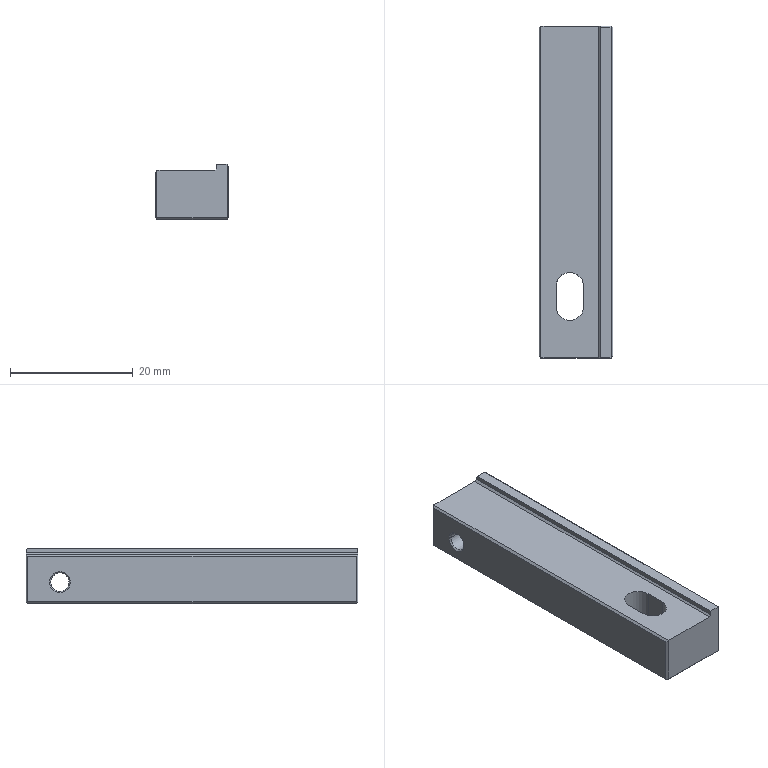Part | NX | 1 solid | 32 faces | box 12 x 54 x 9 mm | volume 4930 mm3 | plane 22 | cylinder 6 | cone 4 | commonest cylinder face diameters 2.5 x2 3 x2 4.5 x2
STEP:
#1=CARTESIAN_POINT('',(2266.8,144.7,-81.));
#2=VERTEX_POINT('',#1);
#3=CARTESIAN_POINT('',(2278.2,144.7,-81.));
#4=VERTEX_POINT('',#3);
#5=CARTESIAN_POINT('',(2272.5,144.7,-81.));
#6=DIRECTION('',(1.,0.,0.));
#7=VECTOR('',#6,1000.);
#8=LINE('',#5,#7);
#9=EDGE_CURVE('',#2,#4,#8,.T.);
#10=ORIENTED_EDGE('',*,*,#9,.T.);
#11=CARTESIAN_POINT('',(2278.2,91.3,-81.));
#12=VERTEX_POINT('',#11);
#13=CARTESIAN_POINT('',(2278.2,118.,-81.));
#14=DIRECTION('',(0.,-1.,0.));
#15=VECTOR('',#14,1000.);
#16=LINE('',#13,#15);
#17=EDGE_CURVE('',#4,#12,#16,.T.);
#18=ORIENTED_EDGE('',*,*,#17,.T.);
#19=CARTESIAN_POINT('',(2266.8,91.3,-81.));
#20=VERTEX_POINT('',#19);
#21=CARTESIAN_POINT('',(2272.5,91.3,-81.));
#22=DIRECTION('',(1.,0.,0.));
#23=VECTOR('',#22,1000.);
#24=LINE('',#21,#23);
#25=EDGE_CURVE('',#20,#12,#24,.T.);
#26=ORIENTED_EDGE('',*,*,#25,.F.);
#27=CARTESIAN_POINT('',(2266.8,118.,-81.));
#28=DIRECTION('',(0.,-1.,0.));
#29=VECTOR('',#28,1000.);
#30=LINE('',#27,#29);
#31=EDGE_CURVE('',#2,#20,#30,.T.);
#32=ORIENTED_EDGE('',*,*,#31,.F.);
#33=EDGE_LOOP('',(#10,#18,#26,#32));
#34=FACE_BOUND('',#33,.T.);
#35=CARTESIAN_POINT('',(2273.75,99.35,-81.));
#36=VERTEX_POINT('',#35);
#37=CARTESIAN_POINT('',(2269.25,99.35,-81.));
#38=VERTEX_POINT('',#37);
#39=CARTESIAN_POINT('',(2271.5,99.35,-81.));
#40=DIRECTION('',(0.,0.,-1.));
#41=DIRECTION('',(-1.,0.,0.));
#42=AXIS2_PLACEMENT_3D('',#39,#40,#41);
#43=CIRCLE('',#42,2.25);
#44=EDGE_CURVE('',#36,#38,#43,.T.);
#45=ORIENTED_EDGE('',*,*,#44,.F.);
#46=CARTESIAN_POINT('',(2273.75,102.65,-81.));
#47=VERTEX_POINT('',#46);
#48=CARTESIAN_POINT('',(2273.75,45.25,-81.));
#49=DIRECTION('',(0.,-1.,0.));
#50=VECTOR('',#49,1000.);
#51=LINE('',#48,#50);
#52=EDGE_CURVE('',#47,#36,#51,.T.);
#53=ORIENTED_EDGE('',*,*,#52,.F.);
#54=CARTESIAN_POINT('',(2269.25,102.65,-81.));
#55=VERTEX_POINT('',#54);
#56=CARTESIAN_POINT('',(2271.5,102.65,-81.));
#57=DIRECTION('',(0.,0.,-1.));
#58=DIRECTION('',(-1.,0.,0.));
#59=AXIS2_PLACEMENT_3D('',#56,#57,#58);
#60=CIRCLE('',#59,2.25);
#61=EDGE_CURVE('',#55,#47,#60,.T.);
#62=ORIENTED_EDGE('',*,*,#61,.F.);
#63=CARTESIAN_POINT('',(2269.25,45.25,-81.));
#64=DIRECTION('',(0.,1.,0.));
#65=VECTOR('',#64,1000.);
#66=LINE('',#63,#65);
#67=EDGE_CURVE('',#38,#55,#66,.T.);
#68=ORIENTED_EDGE('',*,*,#67,.F.);
#69=EDGE_LOOP('',(#45,#53,#62,#68));
#70=FACE_BOUND('',#69,.T.);
#71=CARTESIAN_POINT('',(2266.5,125.,-81.));
#72=DIRECTION('',(0.,0.,-1.));
#73=DIRECTION('',(0.,-1.,0.));
#74=AXIS2_PLACEMENT_3D('',#71,#72,#73);
#75=PLANE('',#74);
#76=ADVANCED_FACE('',(#34,#70),#75,.T.);
#77=CARTESIAN_POINT('',(2278.2,145.,-72.3));
#78=VERTEX_POINT('',#77);
#79=CARTESIAN_POINT('',(2276.5,145.,-72.3));
#80=VERTEX_POINT('',#79);
#81=CARTESIAN_POINT('',(2277.35,145.,-72.3));
#82=DIRECTION('',(-1.,0.,0.));
#83=VECTOR('',#82,1000.);
#84=LINE('',#81,#83);
#85=EDGE_CURVE('',#78,#80,#84,.T.);
#86=ORIENTED_EDGE('',*,*,#85,.F.);
#87=CARTESIAN_POINT('',(2278.2,145.,-80.7));
#88=VERTEX_POINT('',#87);
#89=CARTESIAN_POINT('',(2278.2,145.,-76.5));
#90=DIRECTION('',(0.,0.,-1.));
#91=VECTOR('',#90,1000.);
#92=LINE('',#89,#91);
#93=EDGE_CURVE('',#78,#88,#92,.T.);
#94=ORIENTED_EDGE('',*,*,#93,.T.);
#95=CARTESIAN_POINT('',(2266.8,145.,-80.7));
#96=VERTEX_POINT('',#95);
#97=CARTESIAN_POINT('',(2272.5,145.,-80.7));
#98=DIRECTION('',(1.,0.,0.));
#99=VECTOR('',#98,1000.);
#100=LINE('',#97,#99);
#101=EDGE_CURVE('',#96,#88,#100,.T.);
#102=ORIENTED_EDGE('',*,*,#101,.F.);
#103=CARTESIAN_POINT('',(2266.8,145.,-73.));
#104=VERTEX_POINT('',#103);
#105=CARTESIAN_POINT('',(2266.8,145.,-77.));
#106=DIRECTION('',(0.,0.,-1.));
#107=VECTOR('',#106,1000.);
#108=LINE('',#105,#107);
#109=EDGE_CURVE('',#104,#96,#108,.T.);
#110=ORIENTED_EDGE('',*,*,#109,.F.);
#111=CARTESIAN_POINT('',(2276.2,145.,-73.));
#112=VERTEX_POINT('',#111);
#113=CARTESIAN_POINT('',(2266.5,145.,-73.));
#114=DIRECTION('',(1.,0.,0.));
#115=VECTOR('',#114,1000.);
#116=LINE('',#113,#115);
#117=EDGE_CURVE('',#104,#112,#116,.T.);
#118=ORIENTED_EDGE('',*,*,#117,.T.);
#119=CARTESIAN_POINT('',(2276.5,145.,-72.7));
#120=VERTEX_POINT('',#119);
#121=CARTESIAN_POINT('',(2266.5,145.,-82.7));
#122=DIRECTION('',(0.7071,0.,0.7071));
#123=VECTOR('',#122,1000.);
#124=LINE('',#121,#123);
#125=EDGE_CURVE('',#112,#120,#124,.T.);
#126=ORIENTED_EDGE('',*,*,#125,.T.);
#127=CARTESIAN_POINT('',(2276.5,145.,-12.));
#128=DIRECTION('',(0.,0.,1.));
#129=VECTOR('',#128,1000.);
#130=LINE('',#127,#129);
#131=EDGE_CURVE('',#120,#80,#130,.T.);
#132=ORIENTED_EDGE('',*,*,#131,.T.);
#133=EDGE_LOOP('',(#86,#94,#102,#110,#118,#126,#132));
#134=FACE_BOUND('',#133,.T.);
#135=CARTESIAN_POINT('',(2272.6,145.,-79.2));
#136=VERTEX_POINT('',#135);
#137=CARTESIAN_POINT('',(2272.6,145.,-75.8));
#138=VERTEX_POINT('',#137);
#139=CARTESIAN_POINT('',(2272.6,145.,-77.5));
#140=DIRECTION('',(0.,1.,0.));
#141=DIRECTION('',(0.,0.,1.));
#142=AXIS2_PLACEMENT_3D('',#139,#140,#141);
#143=CIRCLE('',#142,1.7);
#144=EDGE_CURVE('',#136,#138,#143,.T.);
#145=ORIENTED_EDGE('',*,*,#144,.F.);
#146=CARTESIAN_POINT('',(2272.6,145.,-77.5));
#147=DIRECTION('',(0.,1.,0.));
#148=DIRECTION('',(0.,0.,1.));
#149=AXIS2_PLACEMENT_3D('',#146,#147,#148);
#150=CIRCLE('',#149,1.7);
#151=EDGE_CURVE('',#138,#136,#150,.T.);
#152=ORIENTED_EDGE('',*,*,#151,.F.);
#153=EDGE_LOOP('',(#145,#152));
#154=FACE_BOUND('',#153,.T.);
#155=CARTESIAN_POINT('',(2266.5,145.,-72.));
#156=DIRECTION('',(0.,1.,0.));
#157=DIRECTION('',(1.,0.,0.));
#158=AXIS2_PLACEMENT_3D('',#155,#156,#157);
#159=PLANE('',#158);
#160=ADVANCED_FACE('',(#134,#154),#159,.T.);
#161=CARTESIAN_POINT('',(2276.5,91.,-72.));
#162=VERTEX_POINT('',#161);
#163=CARTESIAN_POINT('',(2276.5,144.7,-72.));
#164=VERTEX_POINT('',#163);
#165=CARTESIAN_POINT('',(2276.5,45.25,-72.));
#166=DIRECTION('',(0.,1.,0.));
#167=VECTOR('',#166,1000.);
#168=LINE('',#165,#167);
#169=EDGE_CURVE('',#162,#164,#168,.T.);
#170=ORIENTED_EDGE('',*,*,#169,.F.);
#171=CARTESIAN_POINT('',(2278.2,91.,-72.));
#172=VERTEX_POINT('',#171);
#173=CARTESIAN_POINT('',(2266.5,91.,-72.));
#174=DIRECTION('',(1.,0.,0.));
#175=VECTOR('',#174,1000.);
#176=LINE('',#173,#175);
#177=EDGE_CURVE('',#162,#172,#176,.T.);
#178=ORIENTED_EDGE('',*,*,#177,.T.);
#179=CARTESIAN_POINT('',(2278.2,144.7,-72.));
#180=VERTEX_POINT('',#179);
#181=CARTESIAN_POINT('',(2278.2,118.,-72.));
#182=DIRECTION('',(0.,1.,0.));
#183=VECTOR('',#182,1000.);
#184=LINE('',#181,#183);
#185=EDGE_CURVE('',#172,#180,#184,.T.);
#186=ORIENTED_EDGE('',*,*,#185,.T.);
#187=CARTESIAN_POINT('',(2277.35,144.7,-72.));
#188=DIRECTION('',(-1.,0.,0.));
#189=VECTOR('',#188,1000.);
#190=LINE('',#187,#189);
#191=EDGE_CURVE('',#180,#164,#190,.T.);
#192=ORIENTED_EDGE('',*,*,#191,.T.);
#193=EDGE_LOOP('',(#170,#178,#186,#192));
#194=FACE_BOUND('',#193,.T.);
#195=CARTESIAN_POINT('',(2266.5,91.,-72.));
#196=DIRECTION('',(0.,0.,1.));
#197=DIRECTION('',(1.,0.,0.));
#198=AXIS2_PLACEMENT_3D('',#195,#196,#197);
#199=PLANE('',#198);
#200=ADVANCED_FACE('',(#194),#199,.T.);
#201=CARTESIAN_POINT('',(2276.5,91.,-72.7));
#202=VERTEX_POINT('',#201);
#203=CARTESIAN_POINT('',(2276.5,91.,-12.));
#204=DIRECTION('',(0.,0.,1.));
#205=VECTOR('',#204,1000.);
#206=LINE('',#203,#205);
#207=EDGE_CURVE('',#202,#162,#206,.T.);
#208=ORIENTED_EDGE('',*,*,#207,.F.);
#209=CARTESIAN_POINT('',(2276.2,91.,-73.));
#210=VERTEX_POINT('',#209);
#211=CARTESIAN_POINT('',(2266.5,91.,-82.7));
#212=DIRECTION('',(-0.7071,0.,-0.7071));
#213=VECTOR('',#212,1000.);
#214=LINE('',#211,#213);
#215=EDGE_CURVE('',#202,#210,#214,.T.);
#216=ORIENTED_EDGE('',*,*,#215,.T.);
#217=CARTESIAN_POINT('',(2266.8,91.,-73.));
#218=VERTEX_POINT('',#217);
#219=CARTESIAN_POINT('',(2266.5,91.,-73.));
#220=DIRECTION('',(-1.,0.,0.));
#221=VECTOR('',#220,1000.);
#222=LINE('',#219,#221);
#223=EDGE_CURVE('',#210,#218,#222,.T.);
#224=ORIENTED_EDGE('',*,*,#223,.T.);
#225=CARTESIAN_POINT('',(2266.8,91.,-80.7));
#226=VERTEX_POINT('',#225);
#227=CARTESIAN_POINT('',(2266.8,91.,-77.));
#228=DIRECTION('',(0.,0.,1.));
#229=VECTOR('',#228,1000.);
#230=LINE('',#227,#229);
#231=EDGE_CURVE('',#226,#218,#230,.T.);
#232=ORIENTED_EDGE('',*,*,#231,.F.);
#233=CARTESIAN_POINT('',(2278.2,91.,-80.7));
#234=VERTEX_POINT('',#233);
#235=CARTESIAN_POINT('',(2272.5,91.,-80.7));
#236=DIRECTION('',(1.,0.,0.));
#237=VECTOR('',#236,1000.);
#238=LINE('',#235,#237);
#239=EDGE_CURVE('',#226,#234,#238,.T.);
#240=ORIENTED_EDGE('',*,*,#239,.T.);
#241=CARTESIAN_POINT('',(2278.2,91.,-76.5));
#242=DIRECTION('',(0.,0.,1.));
#243=VECTOR('',#242,1000.);
#244=LINE('',#241,#243);
#245=EDGE_CURVE('',#234,#172,#244,.T.);
#246=ORIENTED_EDGE('',*,*,#245,.T.);
#247=ORIENTED_EDGE('',*,*,#177,.F.);
#248=EDGE_LOOP('',(#208,#216,#224,#232,#240,#246,#247));
#249=FACE_BOUND('',#248,.T.);
#250=CARTESIAN_POINT('',(2266.5,91.,-81.));
#251=DIRECTION('',(0.,-1.,0.));
#252=DIRECTION('',(0.,0.,-1.));
#253=AXIS2_PLACEMENT_3D('',#250,#251,#252);
#254=PLANE('',#253);
#255=ADVANCED_FACE('',(#249),#254,.T.);
#256=CARTESIAN_POINT('',(2276.2,118.,-73.));
#257=DIRECTION('',(0.,-1.,0.));
#258=VECTOR('',#257,1000.);
#259=LINE('',#256,#258);
#260=EDGE_CURVE('',#112,#210,#259,.T.);
#261=ORIENTED_EDGE('',*,*,#260,.F.);
#262=ORIENTED_EDGE('',*,*,#117,.F.);
#263=CARTESIAN_POINT('',(2266.8,118.,-73.));
#264=DIRECTION('',(0.,1.,0.));
#265=VECTOR('',#264,1000.);
#266=LINE('',#263,#265);
#267=EDGE_CURVE('',#218,#104,#266,.T.);
#268=ORIENTED_EDGE('',*,*,#267,.F.);
#269=ORIENTED_EDGE('',*,*,#223,.F.);
#270=EDGE_LOOP('',(#261,#262,#268,#269));
#271=FACE_BOUND('',#270,.T.);
#272=CARTESIAN_POINT('',(2273.75,99.35,-73.));
#273=VERTEX_POINT('',#272);
#274=CARTESIAN_POINT('',(2269.25,99.35,-73.));
#275=VERTEX_POINT('',#274);
#276=CARTESIAN_POINT('',(2271.5,99.35,-73.));
#277=DIRECTION('',(0.,0.,-1.));
#278=DIRECTION('',(-1.,0.,0.));
#279=AXIS2_PLACEMENT_3D('',#276,#277,#278);
#280=CIRCLE('',#279,2.25);
#281=EDGE_CURVE('',#273,#275,#280,.T.);
#282=ORIENTED_EDGE('',*,*,#281,.T.);
#283=CARTESIAN_POINT('',(2269.25,102.65,-73.));
#284=VERTEX_POINT('',#283);
#285=CARTESIAN_POINT('',(2269.25,45.25,-73.));
#286=DIRECTION('',(0.,1.,0.));
#287=VECTOR('',#286,1000.);
#288=LINE('',#285,#287);
#289=EDGE_CURVE('',#275,#284,#288,.T.);
#290=ORIENTED_EDGE('',*,*,#289,.T.);
#291=CARTESIAN_POINT('',(2273.75,102.65,-73.));
#292=VERTEX_POINT('',#291);
#293=CARTESIAN_POINT('',(2271.5,102.65,-73.));
#294=DIRECTION('',(0.,0.,-1.));
#295=DIRECTION('',(-1.,0.,0.));
#296=AXIS2_PLACEMENT_3D('',#293,#294,#295);
#297=CIRCLE('',#296,2.25);
#298=EDGE_CURVE('',#284,#292,#297,.T.);
#299=ORIENTED_EDGE('',*,*,#298,.T.);
#300=CARTESIAN_POINT('',(2273.75,45.25,-73.));
#301=DIRECTION('',(0.,-1.,0.));
#302=VECTOR('',#301,1000.);
#303=LINE('',#300,#302);
#304=EDGE_CURVE('',#292,#273,#303,.T.);
#305=ORIENTED_EDGE('',*,*,#304,.T.);
#306=EDGE_LOOP('',(#282,#290,#299,#305));
#307=FACE_BOUND('',#306,.T.);
#308=CARTESIAN_POINT('',(2275.402,98.391,-73.));
#309=DIRECTION('',(0.,0.,1.));
#310=DIRECTION('',(1.,0.,0.));
#311=AXIS2_PLACEMENT_3D('',#308,#309,#310);
#312=PLANE('',#311);
#313=ADVANCED_FACE('',(#271,#307),#312,.T.);
#314=ORIENTED_EDGE('',*,*,#131,.F.);
#315=CARTESIAN_POINT('',(2276.5,118.,-72.7));
#316=DIRECTION('',(0.,-1.,0.));
#317=VECTOR('',#316,1000.);
#318=LINE('',#315,#317);
#319=EDGE_CURVE('',#120,#202,#318,.T.);
#320=ORIENTED_EDGE('',*,*,#319,.T.);
#321=ORIENTED_EDGE('',*,*,#207,.T.);
#322=ORIENTED_EDGE('',*,*,#169,.T.);
#323=CARTESIAN_POINT('',(2276.5,84.7,-12.));
#324=DIRECTION('',(0.,-0.7071,0.7071));
#325=VECTOR('',#324,1000.);
#326=LINE('',#323,#325);
#327=EDGE_CURVE('',#80,#164,#326,.T.);
#328=ORIENTED_EDGE('',*,*,#327,.F.);
#329=EDGE_LOOP('',(#314,#320,#321,#322,#328));
#330=FACE_BOUND('',#329,.T.);
#331=CARTESIAN_POINT('',(2276.5,91.,-72.));
#332=DIRECTION('',(1.,0.,0.));
#333=DIRECTION('',(0.,1.,0.));
#334=AXIS2_PLACEMENT_3D('',#331,#332,#333);
#335=PLANE('',#334);
#336=ADVANCED_FACE('',(#330),#335,.F.);
#337=ORIENTED_EDGE('',*,*,#281,.F.);
#338=CARTESIAN_POINT('',(2273.75,99.35,-71.1));
#339=DIRECTION('',(0.,0.,-1.));
#340=VECTOR('',#339,1000.);
#341=LINE('',#338,#340);
#342=EDGE_CURVE('',#273,#36,#341,.T.);
#343=ORIENTED_EDGE('',*,*,#342,.T.);
#344=ORIENTED_EDGE('',*,*,#44,.T.);
#345=CARTESIAN_POINT('',(2269.25,99.35,-71.1));
#346=DIRECTION('',(0.,0.,-1.));
#347=VECTOR('',#346,1000.);
#348=LINE('',#345,#347);
#349=EDGE_CURVE('',#275,#38,#348,.T.);
#350=ORIENTED_EDGE('',*,*,#349,.F.);
#351=EDGE_LOOP('',(#337,#343,#344,#350));
#352=FACE_BOUND('',#351,.T.);
#353=CARTESIAN_POINT('',(2271.5,99.35,-71.1));
#354=DIRECTION('',(0.,0.,-1.));
#355=DIRECTION('',(-1.,0.,0.));
#356=AXIS2_PLACEMENT_3D('',#353,#354,#355);
#357=CYLINDRICAL_SURFACE('',#356,2.25);
#358=ADVANCED_FACE('',(#352),#357,.F.);
#359=ORIENTED_EDGE('',*,*,#304,.F.);
#360=CARTESIAN_POINT('',(2273.75,102.65,-71.1));
#361=DIRECTION('',(0.,0.,-1.));
#362=VECTOR('',#361,1000.);
#363=LINE('',#360,#362);
#364=EDGE_CURVE('',#292,#47,#363,.T.);
#365=ORIENTED_EDGE('',*,*,#364,.T.);
#366=ORIENTED_EDGE('',*,*,#52,.T.);
#367=ORIENTED_EDGE('',*,*,#342,.F.);
#368=EDGE_LOOP('',(#359,#365,#366,#367));
#369=FACE_BOUND('',#368,.T.);
#370=CARTESIAN_POINT('',(2273.75,99.35,-71.1));
#371=DIRECTION('',(1.,0.,0.));
#372=DIRECTION('',(0.,1.,0.));
#373=AXIS2_PLACEMENT_3D('',#370,#371,#372);
#374=PLANE('',#373);
#375=ADVANCED_FACE('',(#369),#374,.F.);
#376=ORIENTED_EDGE('',*,*,#298,.F.);
#377=CARTESIAN_POINT('',(2269.25,102.65,-71.1));
#378=DIRECTION('',(0.,0.,-1.));
#379=VECTOR('',#378,1000.);
#380=LINE('',#377,#379);
#381=EDGE_CURVE('',#284,#55,#380,.T.);
#382=ORIENTED_EDGE('',*,*,#381,.T.);
#383=ORIENTED_EDGE('',*,*,#61,.T.);
#384=ORIENTED_EDGE('',*,*,#364,.F.);
#385=EDGE_LOOP('',(#376,#382,#383,#384));
#386=FACE_BOUND('',#385,.T.);
#387=CARTESIAN_POINT('',(2271.5,102.65,-71.1));
#388=DIRECTION('',(0.,0.,-1.));
#389=DIRECTION('',(-1.,0.,0.));
#390=AXIS2_PLACEMENT_3D('',#387,#388,#389);
#391=CYLINDRICAL_SURFACE('',#390,2.25);
#392=ADVANCED_FACE('',(#386),#391,.F.);
#393=ORIENTED_EDGE('',*,*,#289,.F.);
#394=ORIENTED_EDGE('',*,*,#349,.T.);
#395=ORIENTED_EDGE('',*,*,#67,.T.);
#396=ORIENTED_EDGE('',*,*,#381,.F.);
#397=EDGE_LOOP('',(#393,#394,#395,#396));
#398=FACE_BOUND('',#397,.T.);
#399=CARTESIAN_POINT('',(2269.25,102.65,-71.1));
#400=DIRECTION('',(-1.,0.,0.));
#401=DIRECTION('',(0.,0.,1.));
#402=AXIS2_PLACEMENT_3D('',#399,#400,#401);
#403=PLANE('',#402);
#404=ADVANCED_FACE('',(#398),#403,.F.);
#405=CARTESIAN_POINT('',(2272.6,144.74,-78.75));
#406=VERTEX_POINT('',#405);
#407=CARTESIAN_POINT('',(2272.6,144.74,-76.25));
#408=VERTEX_POINT('',#407);
#409=CARTESIAN_POINT('',(2272.6,144.74,-77.5));
#410=DIRECTION('',(0.,1.,0.));
#411=DIRECTION('',(0.,0.,1.));
#412=AXIS2_PLACEMENT_3D('',#409,#410,#411);
#413=CIRCLE('',#412,1.25);
#414=EDGE_CURVE('',#406,#408,#413,.T.);
#415=ORIENTED_EDGE('',*,*,#414,.T.);
#416=CARTESIAN_POINT('',(2272.6,140.329,-76.25));
#417=VERTEX_POINT('',#416);
#418=CARTESIAN_POINT('',(2272.6,145.,-76.25));
#419=DIRECTION('',(0.,1.,0.));
#420=VECTOR('',#419,1000.);
#421=LINE('',#418,#420);
#422=EDGE_CURVE('',#408,#417,#421,.F.);
#423=ORIENTED_EDGE('',*,*,#422,.T.);
#424=CARTESIAN_POINT('',(2271.35,141.,-77.5));
#425=VERTEX_POINT('',#424);
#426=CARTESIAN_POINT('',(2271.35,141.,-77.5));
#427=CARTESIAN_POINT('',(2271.35,141.,-77.478));
#428=CARTESIAN_POINT('',(2271.351,141.,-77.456));
#429=CARTESIAN_POINT('',(2271.352,140.999,-77.434));
#430=CARTESIAN_POINT('',(2271.353,140.998,-77.413));
#431=CARTESIAN_POINT('',(2271.355,140.996,-77.391));
#432=CARTESIAN_POINT('',(2271.357,140.994,-77.369));
#433=CARTESIAN_POINT('',(2271.359,140.992,-77.348));
#434=CARTESIAN_POINT('',(2271.362,140.99,-77.326));
#435=CARTESIAN_POINT('',(2271.365,140.987,-77.305));
#436=CARTESIAN_POINT('',(2271.369,140.984,-77.284));
#437=CARTESIAN_POINT('',(2271.373,140.981,-77.262));
#438=CARTESIAN_POINT('',(2271.377,140.977,-77.241));
#439=CARTESIAN_POINT('',(2271.382,140.974,-77.22));
#440=CARTESIAN_POINT('',(2271.387,140.97,-77.199));
#441=CARTESIAN_POINT('',(2271.392,140.965,-77.178));
#442=CARTESIAN_POINT('',(2271.398,140.961,-77.158));
#443=CARTESIAN_POINT('',(2271.404,140.956,-77.137));
#444=CARTESIAN_POINT('',(2271.41,140.95,-77.117));
#445=CARTESIAN_POINT('',(2271.417,140.945,-77.097));
#446=CARTESIAN_POINT('',(2271.424,140.939,-77.077));
#447=CARTESIAN_POINT('',(2271.431,140.933,-77.057));
#448=CARTESIAN_POINT('',(2271.438,140.927,-77.038));
#449=CARTESIAN_POINT('',(2271.446,140.921,-77.019));
#450=CARTESIAN_POINT('',(2271.455,140.914,-77.));
#451=CARTESIAN_POINT('',(2271.463,140.907,-76.981));
#452=CARTESIAN_POINT('',(2271.472,140.9,-76.962));
#453=CARTESIAN_POINT('',(2271.481,140.893,-76.943));
#454=CARTESIAN_POINT('',(2271.49,140.886,-76.925));
#455=CARTESIAN_POINT('',(2271.499,140.878,-76.907));
#456=CARTESIAN_POINT('',(2271.509,140.87,-76.889));
#457=CARTESIAN_POINT('',(2271.519,140.862,-76.871));
#458=CARTESIAN_POINT('',(2271.53,140.854,-76.854));
#459=CARTESIAN_POINT('',(2271.541,140.845,-76.837));
#460=CARTESIAN_POINT('',(2271.551,140.837,-76.819));
#461=CARTESIAN_POINT('',(2271.562,140.828,-76.803));
#462=CARTESIAN_POINT('',(2271.574,140.819,-76.786));
#463=CARTESIAN_POINT('',(2271.585,140.81,-76.77));
#464=CARTESIAN_POINT('',(2271.597,140.801,-76.754));
#465=CARTESIAN_POINT('',(2271.609,140.792,-76.738));
#466=CARTESIAN_POINT('',(2271.621,140.783,-76.722));
#467=CARTESIAN_POINT('',(2271.633,140.773,-76.707));
#468=CARTESIAN_POINT('',(2271.646,140.764,-76.692));
#469=CARTESIAN_POINT('',(2271.671,140.745,-76.662));
#470=CARTESIAN_POINT('',(2271.698,140.725,-76.634));
#471=CARTESIAN_POINT('',(2271.726,140.705,-76.607));
#472=CARTESIAN_POINT('',(2271.753,140.685,-76.579));
#473=CARTESIAN_POINT('',(2271.782,140.664,-76.554));
#474=CARTESIAN_POINT('',(2271.812,140.644,-76.529));
#475=CARTESIAN_POINT('',(2271.827,140.633,-76.517));
#476=CARTESIAN_POINT('',(2271.843,140.623,-76.505));
#477=CARTESIAN_POINT('',(2271.858,140.612,-76.494));
#478=CARTESIAN_POINT('',(2271.874,140.602,-76.482));
#479=CARTESIAN_POINT('',(2271.89,140.592,-76.471));
#480=CARTESIAN_POINT('',(2271.906,140.581,-76.46));
#481=CARTESIAN_POINT('',(2271.922,140.571,-76.45));
#482=CARTESIAN_POINT('',(2271.938,140.561,-76.439));
#483=CARTESIAN_POINT('',(2271.955,140.551,-76.429));
#484=CARTESIAN_POINT('',(2271.971,140.54,-76.419));
#485=CARTESIAN_POINT('',(2271.988,140.53,-76.41));
#486=CARTESIAN_POINT('',(2272.005,140.52,-76.401));
#487=CARTESIAN_POINT('',(2272.022,140.51,-76.391));
#488=CARTESIAN_POINT('',(2272.04,140.501,-76.382));
#489=CARTESIAN_POINT('',(2272.057,140.491,-76.374));
#490=CARTESIAN_POINT('',(2272.075,140.481,-76.366));
#491=CARTESIAN_POINT('',(2272.093,140.472,-76.357));
#492=CARTESIAN_POINT('',(2272.111,140.463,-76.35));
#493=CARTESIAN_POINT('',(2272.129,140.453,-76.342));
#494=CARTESIAN_POINT('',(2272.148,140.444,-76.335));
#495=CARTESIAN_POINT('',(2272.167,140.436,-76.328));
#496=CARTESIAN_POINT('',(2272.185,140.427,-76.321));
#497=CARTESIAN_POINT('',(2272.204,140.418,-76.314));
#498=CARTESIAN_POINT('',(2272.224,140.41,-76.308));
#499=CARTESIAN_POINT('',(2272.263,140.394,-76.296));
#500=CARTESIAN_POINT('',(2272.303,140.38,-76.285));
#501=CARTESIAN_POINT('',(2272.343,140.368,-76.277));
#502=CARTESIAN_POINT('',(2272.364,140.362,-76.272));
#503=CARTESIAN_POINT('',(2272.385,140.356,-76.269));
#504=CARTESIAN_POINT('',(2272.406,140.352,-76.265));
#505=CARTESIAN_POINT('',(2272.427,140.347,-76.262));
#506=CARTESIAN_POINT('',(2272.448,140.343,-76.259));
#507=CARTESIAN_POINT('',(2272.47,140.339,-76.257));
#508=CARTESIAN_POINT('',(2272.48,140.338,-76.256));
#509=CARTESIAN_POINT('',(2272.491,140.336,-76.255));
#510=CARTESIAN_POINT('',(2272.502,140.335,-76.254));
#511=CARTESIAN_POINT('',(2272.513,140.334,-76.253));
#512=CARTESIAN_POINT('',(2272.524,140.333,-76.252));
#513=CARTESIAN_POINT('',(2272.535,140.332,-76.252));
#514=CARTESIAN_POINT('',(2272.546,140.331,-76.251));
#515=CARTESIAN_POINT('',(2272.556,140.33,-76.251));
#516=CARTESIAN_POINT('',(2272.567,140.33,-76.25));
#517=CARTESIAN_POINT('',(2272.578,140.329,-76.25));
#518=CARTESIAN_POINT('',(2272.589,140.329,-76.25));
#519=CARTESIAN_POINT('',(2272.6,140.329,-76.25));
#520=B_SPLINE_CURVE_WITH_KNOTS('',3,(#426,#427,#428,#429,#430,#431,#432,#433,#434,#435,#436,#437,#438,#439,#440,#441,#442,#443,#444,#445,#446,#447,#448,#449,#450,#451,#452,#453,#454,#455,#456,#457,#458,#459,#460,#461,#462,#463,#464,#465,#466,#467,#468,#469,#470,#471,#472,#473,#474,#475,#476,#477,#478,#479,#480,#481,#482,#483,#484,#485,#486,#487,#488,#489,#490,#491,#492,#493,#494,#495,#496,#497,#498,#499,#500,#501,#502,#503,#504,#505,#506,#507,#508,#509,#510,#511,#512,#513,#514,#515,#516,#517,#518,#519),.UNSPECIFIED.,.F.,.F.,(4,3,3,3,3,3,3,3,3,3,3,3,3,3,3,3,3,3,3,3,3,3,3,3,3,3,3,3,3,3,3,4),(0.,0.06563,0.131,0.1964,0.262,0.3277,0.3934,0.4588,0.5241,0.5896,0.6553,0.721,0.7868,0.8524,0.9178,1.049,1.18,1.246,1.312,1.377,1.443,1.508,1.574,1.639,1.705,1.836,1.901,1.967,2.,2.033,2.065,2.098),.UNSPECIFIED.);
#521=EDGE_CURVE('',#425,#417,#520,.T.);
#522=ORIENTED_EDGE('',*,*,#521,.F.);
#523=CARTESIAN_POINT('',(2272.6,140.329,-78.75));
#524=VERTEX_POINT('',#523);
#525=CARTESIAN_POINT('',(2272.6,140.329,-78.75));
#526=CARTESIAN_POINT('',(2272.589,140.329,-78.75));
#527=CARTESIAN_POINT('',(2272.578,140.329,-78.75));
#528=CARTESIAN_POINT('',(2272.567,140.33,-78.75));
#529=CARTESIAN_POINT('',(2272.556,140.33,-78.749));
#530=CARTESIAN_POINT('',(2272.545,140.331,-78.749));
#531=CARTESIAN_POINT('',(2272.534,140.332,-78.748));
#532=CARTESIAN_POINT('',(2272.523,140.333,-78.748));
#533=CARTESIAN_POINT('',(2272.512,140.334,-78.747));
#534=CARTESIAN_POINT('',(2272.502,140.335,-78.746));
#535=CARTESIAN_POINT('',(2272.491,140.336,-78.745));
#536=CARTESIAN_POINT('',(2272.48,140.338,-78.744));
#537=CARTESIAN_POINT('',(2272.469,140.339,-78.743));
#538=CARTESIAN_POINT('',(2272.448,140.343,-78.741));
#539=CARTESIAN_POINT('',(2272.427,140.347,-78.738));
#540=CARTESIAN_POINT('',(2272.406,140.352,-78.735));
#541=CARTESIAN_POINT('',(2272.385,140.356,-78.732));
#542=CARTESIAN_POINT('',(2272.364,140.362,-78.728));
#543=CARTESIAN_POINT('',(2272.343,140.368,-78.723));
#544=CARTESIAN_POINT('',(2272.323,140.374,-78.719));
#545=CARTESIAN_POINT('',(2272.303,140.381,-78.714));
#546=CARTESIAN_POINT('',(2272.283,140.388,-78.709));
#547=CARTESIAN_POINT('',(2272.263,140.395,-78.704));
#548=CARTESIAN_POINT('',(2272.243,140.403,-78.698));
#549=CARTESIAN_POINT('',(2272.223,140.411,-78.692));
#550=CARTESIAN_POINT('',(2272.204,140.419,-78.686));
#551=CARTESIAN_POINT('',(2272.185,140.427,-78.679));
#552=CARTESIAN_POINT('',(2272.166,140.436,-78.672));
#553=CARTESIAN_POINT('',(2272.148,140.444,-78.665));
#554=CARTESIAN_POINT('',(2272.129,140.453,-78.658));
#555=CARTESIAN_POINT('',(2272.111,140.463,-78.65));
#556=CARTESIAN_POINT('',(2272.093,140.472,-78.643));
#557=CARTESIAN_POINT('',(2272.075,140.481,-78.635));
#558=CARTESIAN_POINT('',(2272.057,140.491,-78.626));
#559=CARTESIAN_POINT('',(2272.04,140.501,-78.618));
#560=CARTESIAN_POINT('',(2272.022,140.51,-78.609));
#561=CARTESIAN_POINT('',(2272.005,140.52,-78.599));
#562=CARTESIAN_POINT('',(2271.988,140.53,-78.59));
#563=CARTESIAN_POINT('',(2271.971,140.541,-78.581));
#564=CARTESIAN_POINT('',(2271.955,140.551,-78.571));
#565=CARTESIAN_POINT('',(2271.938,140.561,-78.561));
#566=CARTESIAN_POINT('',(2271.922,140.571,-78.55));
#567=CARTESIAN_POINT('',(2271.906,140.581,-78.539));
#568=CARTESIAN_POINT('',(2271.89,140.592,-78.529));
#569=CARTESIAN_POINT('',(2271.874,140.602,-78.518));
#570=CARTESIAN_POINT('',(2271.858,140.612,-78.506));
#571=CARTESIAN_POINT('',(2271.843,140.623,-78.495));
#572=CARTESIAN_POINT('',(2271.828,140.633,-78.483));
#573=CARTESIAN_POINT('',(2271.813,140.643,-78.471));
#574=CARTESIAN_POINT('',(2271.783,140.664,-78.447));
#575=CARTESIAN_POINT('',(2271.754,140.684,-78.421));
#576=CARTESIAN_POINT('',(2271.726,140.704,-78.394));
#577=CARTESIAN_POINT('',(2271.699,140.725,-78.367));
#578=CARTESIAN_POINT('',(2271.672,140.744,-78.338));
#579=CARTESIAN_POINT('',(2271.646,140.764,-78.308));
#580=CARTESIAN_POINT('',(2271.621,140.783,-78.278));
#581=CARTESIAN_POINT('',(2271.597,140.802,-78.247));
#582=CARTESIAN_POINT('',(2271.574,140.819,-78.214));
#583=CARTESIAN_POINT('',(2271.551,140.837,-78.181));
#584=CARTESIAN_POINT('',(2271.53,140.854,-78.147));
#585=CARTESIAN_POINT('',(2271.51,140.87,-78.111));
#586=CARTESIAN_POINT('',(2271.49,140.885,-78.076));
#587=CARTESIAN_POINT('',(2271.472,140.9,-78.039));
#588=CARTESIAN_POINT('',(2271.455,140.914,-78.001));
#589=CARTESIAN_POINT('',(2271.447,140.921,-77.982));
#590=CARTESIAN_POINT('',(2271.439,140.927,-77.963));
#591=CARTESIAN_POINT('',(2271.431,140.933,-77.943));
#592=CARTESIAN_POINT('',(2271.424,140.939,-77.923));
#593=CARTESIAN_POINT('',(2271.417,140.945,-77.903));
#594=CARTESIAN_POINT('',(2271.41,140.95,-77.883));
#595=CARTESIAN_POINT('',(2271.404,140.956,-77.863));
#596=CARTESIAN_POINT('',(2271.398,140.961,-77.842));
#597=CARTESIAN_POINT('',(2271.392,140.965,-77.822));
#598=CARTESIAN_POINT('',(2271.387,140.97,-77.801));
#599=CARTESIAN_POINT('',(2271.382,140.974,-77.78));
#600=CARTESIAN_POINT('',(2271.377,140.977,-77.759));
#601=CARTESIAN_POINT('',(2271.373,140.981,-77.738));
#602=CARTESIAN_POINT('',(2271.369,140.984,-77.717));
#603=CARTESIAN_POINT('',(2271.365,140.987,-77.695));
#604=CARTESIAN_POINT('',(2271.362,140.99,-77.674));
#605=CARTESIAN_POINT('',(2271.359,140.992,-77.653));
#606=CARTESIAN_POINT('',(2271.357,140.994,-77.631));
#607=CARTESIAN_POINT('',(2271.355,140.996,-77.609));
#608=CARTESIAN_POINT('',(2271.353,140.998,-77.588));
#609=CARTESIAN_POINT('',(2271.352,140.999,-77.566));
#610=CARTESIAN_POINT('',(2271.351,141.,-77.544));
#611=CARTESIAN_POINT('',(2271.35,141.,-77.522));
#612=CARTESIAN_POINT('',(2271.35,141.,-77.5));
#613=B_SPLINE_CURVE_WITH_KNOTS('',3,(#525,#526,#527,#528,#529,#530,#531,#532,#533,#534,#535,#536,#537,#538,#539,#540,#541,#542,#543,#544,#545,#546,#547,#548,#549,#550,#551,#552,#553,#554,#555,#556,#557,#558,#559,#560,#561,#562,#563,#564,#565,#566,#567,#568,#569,#570,#571,#572,#573,#574,#575,#576,#577,#578,#579,#580,#581,#582,#583,#584,#585,#586,#587,#588,#589,#590,#591,#592,#593,#594,#595,#596,#597,#598,#599,#600,#601,#602,#603,#604,#605,#606,#607,#608,#609,#610,#611,#612),.UNSPECIFIED.,.F.,.F.,(4,3,3,3,3,3,3,3,3,3,3,3,3,3,3,3,3,3,3,3,3,3,3,3,3,3,3,3,3,4),(0.,0.03292,0.06582,0.09866,0.1314,0.1967,0.2622,0.3278,0.3934,0.4588,0.5241,0.5895,0.6551,0.7207,0.7864,0.8519,0.9173,1.048,1.18,1.311,1.442,1.573,1.639,1.705,1.77,1.836,1.901,1.967,2.032,2.098),.UNSPECIFIED.);
#614=EDGE_CURVE('',#524,#425,#613,.T.);
#615=ORIENTED_EDGE('',*,*,#614,.F.);
#616=CARTESIAN_POINT('',(2272.6,145.,-78.75));
#617=DIRECTION('',(0.,1.,0.));
#618=VECTOR('',#617,1000.);
#619=LINE('',#616,#618);
#620=EDGE_CURVE('',#406,#524,#619,.F.);
#621=ORIENTED_EDGE('',*,*,#620,.F.);
#622=EDGE_LOOP('',(#415,#423,#522,#615,#621));
#623=FACE_BOUND('',#622,.T.);
#624=CARTESIAN_POINT('',(2272.6,145.,-77.5));
#625=DIRECTION('',(0.,1.,0.));
#626=DIRECTION('',(0.,0.,1.));
#627=AXIS2_PLACEMENT_3D('',#624,#625,#626);
#628=CYLINDRICAL_SURFACE('',#627,1.25);
#629=ADVANCED_FACE('',(#623),#628,.F.);
#630=ORIENTED_EDGE('',*,*,#414,.F.);
#631=CARTESIAN_POINT('',(2272.6,144.74,-78.75));
#632=DIRECTION('',(0.,0.5,-0.866));
#633=VECTOR('',#632,1000.);
#634=LINE('',#631,#633);
#635=EDGE_CURVE('',#406,#136,#634,.T.);
#636=ORIENTED_EDGE('',*,*,#635,.T.);
#637=ORIENTED_EDGE('',*,*,#144,.T.);
#638=CARTESIAN_POINT('',(2272.6,144.74,-76.25));
#639=DIRECTION('',(0.,0.5,0.866));
#640=VECTOR('',#639,1000.);
#641=LINE('',#638,#640);
#642=EDGE_CURVE('',#408,#138,#641,.T.);
#643=ORIENTED_EDGE('',*,*,#642,.F.);
#644=EDGE_LOOP('',(#630,#636,#637,#643));
#645=FACE_BOUND('',#644,.T.);
#646=CARTESIAN_POINT('',(2272.6,144.74,-77.5));
#647=DIRECTION('',(0.,1.,0.));
#648=DIRECTION('',(0.,0.,1.));
#649=AXIS2_PLACEMENT_3D('',#646,#647,#648);
#650=CONICAL_SURFACE('',#649,1.25,1.047);
#651=ADVANCED_FACE('',(#645),#650,.F.);
#652=ORIENTED_EDGE('',*,*,#25,.T.);
#653=CARTESIAN_POINT('',(2278.35,91.15,-80.85));
#654=VERTEX_POINT('',#653);
#655=CARTESIAN_POINT('',(2266.5,103.,-92.7));
#656=DIRECTION('',(0.5774,-0.5774,0.5774));
#657=VECTOR('',#656,1000.);
#658=LINE('',#655,#657);
#659=EDGE_CURVE('',#12,#654,#658,.T.);
#660=ORIENTED_EDGE('',*,*,#659,.T.);
#661=CARTESIAN_POINT('',(2266.5,79.3,-69.));
#662=DIRECTION('',(-0.5774,-0.5774,0.5774));
#663=VECTOR('',#662,1000.);
#664=LINE('',#661,#663);
#665=EDGE_CURVE('',#654,#234,#664,.T.);
#666=ORIENTED_EDGE('',*,*,#665,.T.);
#667=ORIENTED_EDGE('',*,*,#239,.F.);
#668=CARTESIAN_POINT('',(2266.65,91.15,-80.85));
#669=VERTEX_POINT('',#668);
#670=CARTESIAN_POINT('',(2266.5,91.3,-81.));
#671=DIRECTION('',(0.5774,-0.5774,0.5774));
#672=VECTOR('',#671,1000.);
#673=LINE('',#670,#672);
#674=EDGE_CURVE('',#669,#226,#673,.T.);
#675=ORIENTED_EDGE('',*,*,#674,.F.);
#676=CARTESIAN_POINT('',(2266.5,91.,-80.7));
#677=DIRECTION('',(-0.5774,-0.5774,0.5774));
#678=VECTOR('',#677,1000.);
#679=LINE('',#676,#678);
#680=EDGE_CURVE('',#20,#669,#679,.T.);
#681=ORIENTED_EDGE('',*,*,#680,.F.);
#682=EDGE_LOOP('',(#652,#660,#666,#667,#675,#681));
#683=FACE_BOUND('',#682,.T.);
#684=CARTESIAN_POINT('',(2272.5,91.15,-80.85));
#685=DIRECTION('',(0.,0.7071,0.7071));
#686=DIRECTION('',(1.,0.,0.));
#687=AXIS2_PLACEMENT_3D('',#684,#685,#686);
#688=PLANE('',#687);
#689=ADVANCED_FACE('',(#683),#688,.F.);
#690=ORIENTED_EDGE('',*,*,#267,.T.);
#691=CARTESIAN_POINT('',(2266.5,144.7,-73.3));
#692=VERTEX_POINT('',#691);
#693=CARTESIAN_POINT('',(2266.5,144.7,-73.3));
#694=DIRECTION('',(0.5774,0.5774,0.5774));
#695=VECTOR('',#694,1000.);
#696=LINE('',#693,#695);
#697=EDGE_CURVE('',#692,#104,#696,.T.);
#698=ORIENTED_EDGE('',*,*,#697,.F.);
#699=CARTESIAN_POINT('',(2266.5,91.3,-73.3));
#700=VERTEX_POINT('',#699);
#701=CARTESIAN_POINT('',(2266.5,118.,-73.3));
#702=DIRECTION('',(0.,1.,0.));
#703=VECTOR('',#702,1000.);
#704=LINE('',#701,#703);
#705=EDGE_CURVE('',#700,#692,#704,.T.);
#706=ORIENTED_EDGE('',*,*,#705,.F.);
#707=CARTESIAN_POINT('',(2266.5,91.3,-73.3));
#708=DIRECTION('',(-0.5774,0.5774,-0.5774));
#709=VECTOR('',#708,1000.);
#710=LINE('',#707,#709);
#711=EDGE_CURVE('',#218,#700,#710,.T.);
#712=ORIENTED_EDGE('',*,*,#711,.F.);
#713=EDGE_LOOP('',(#690,#698,#706,#712));
#714=FACE_BOUND('',#713,.T.);
#715=CARTESIAN_POINT('',(2266.65,118.,-73.15));
#716=DIRECTION('',(0.7071,0.,-0.7071));
#717=DIRECTION('',(0.,-1.,0.));
#718=AXIS2_PLACEMENT_3D('',#715,#716,#717);
#719=PLANE('',#718);
#720=ADVANCED_FACE('',(#714),#719,.F.);
#721=ORIENTED_EDGE('',*,*,#260,.T.);
#722=ORIENTED_EDGE('',*,*,#215,.F.);
#723=ORIENTED_EDGE('',*,*,#319,.F.);
#724=ORIENTED_EDGE('',*,*,#125,.F.);
#725=EDGE_LOOP('',(#721,#722,#723,#724));
#726=FACE_BOUND('',#725,.T.);
#727=CARTESIAN_POINT('',(2276.35,118.,-72.85));
#728=DIRECTION('',(0.7071,0.,-0.7071));
#729=DIRECTION('',(0.,-1.,0.));
#730=AXIS2_PLACEMENT_3D('',#727,#728,#729);
#731=PLANE('',#730);
#732=ADVANCED_FACE('',(#726),#731,.F.);
#733=ORIENTED_EDGE('',*,*,#9,.F.);
#734=CARTESIAN_POINT('',(2266.65,144.85,-80.85));
#735=VERTEX_POINT('',#734);
#736=CARTESIAN_POINT('',(2266.5,145.,-80.7));
#737=DIRECTION('',(0.5774,-0.5774,-0.5774));
#738=VECTOR('',#737,1000.);
#739=LINE('',#736,#738);
#740=EDGE_CURVE('',#735,#2,#739,.T.);
#741=ORIENTED_EDGE('',*,*,#740,.F.);
#742=CARTESIAN_POINT('',(2266.5,144.7,-81.));
#743=DIRECTION('',(0.5774,0.5774,0.5774));
#744=VECTOR('',#743,1000.);
#745=LINE('',#742,#744);
#746=EDGE_CURVE('',#735,#96,#745,.T.);
#747=ORIENTED_EDGE('',*,*,#746,.T.);
#748=ORIENTED_EDGE('',*,*,#101,.T.);
#749=CARTESIAN_POINT('',(2278.35,144.85,-80.85));
#750=VERTEX_POINT('',#749);
#751=CARTESIAN_POINT('',(2266.5,156.7,-69.));
#752=DIRECTION('',(-0.5774,0.5774,0.5774));
#753=VECTOR('',#752,1000.);
#754=LINE('',#751,#753);
#755=EDGE_CURVE('',#750,#88,#754,.T.);
#756=ORIENTED_EDGE('',*,*,#755,.F.);
#757=CARTESIAN_POINT('',(2266.5,133.,-92.7));
#758=DIRECTION('',(-0.5774,-0.5774,-0.5774));
#759=VECTOR('',#758,1000.);
#760=LINE('',#757,#759);
#761=EDGE_CURVE('',#750,#4,#760,.T.);
#762=ORIENTED_EDGE('',*,*,#761,.T.);
#763=EDGE_LOOP('',(#733,#741,#747,#748,#756,#762));
#764=FACE_BOUND('',#763,.T.);
#765=CARTESIAN_POINT('',(2272.5,144.85,-80.85));
#766=DIRECTION('',(0.,0.7071,-0.7071));
#767=DIRECTION('',(-1.,0.,0.));
#768=AXIS2_PLACEMENT_3D('',#765,#766,#767);
#769=PLANE('',#768);
#770=ADVANCED_FACE('',(#764),#769,.T.);
#771=ORIENTED_EDGE('',*,*,#85,.T.);
#772=ORIENTED_EDGE('',*,*,#327,.T.);
#773=ORIENTED_EDGE('',*,*,#191,.F.);
#774=CARTESIAN_POINT('',(2278.35,144.85,-72.15));
#775=VERTEX_POINT('',#774);
#776=CARTESIAN_POINT('',(2266.5,133.,-60.3));
#777=DIRECTION('',(0.5774,0.5774,-0.5774));
#778=VECTOR('',#777,1000.);
#779=LINE('',#776,#778);
#780=EDGE_CURVE('',#180,#775,#779,.T.);
#781=ORIENTED_EDGE('',*,*,#780,.T.);
#782=CARTESIAN_POINT('',(2266.5,156.7,-84.));
#783=DIRECTION('',(-0.5774,0.5774,-0.5774));
#784=VECTOR('',#783,1000.);
#785=LINE('',#782,#784);
#786=EDGE_CURVE('',#775,#78,#785,.T.);
#787=ORIENTED_EDGE('',*,*,#786,.T.);
#788=EDGE_LOOP('',(#771,#772,#773,#781,#787));
#789=FACE_BOUND('',#788,.T.);
#790=CARTESIAN_POINT('',(2277.35,144.85,-72.15));
#791=DIRECTION('',(0.,-0.7071,-0.7071));
#792=DIRECTION('',(0.,-0.7071,0.7071));
#793=AXIS2_PLACEMENT_3D('',#790,#791,#792);
#794=PLANE('',#793);
#795=ADVANCED_FACE('',(#789),#794,.F.);
#796=ORIENTED_EDGE('',*,*,#620,.T.);
#797=CARTESIAN_POINT('',(2273.85,141.,-77.5));
#798=VERTEX_POINT('',#797);
#799=CARTESIAN_POINT('',(2273.85,141.,-77.5));
#800=CARTESIAN_POINT('',(2273.85,141.,-77.522));
#801=CARTESIAN_POINT('',(2273.849,141.,-77.544));
#802=CARTESIAN_POINT('',(2273.848,140.999,-77.566));
#803=CARTESIAN_POINT('',(2273.847,140.998,-77.587));
#804=CARTESIAN_POINT('',(2273.845,140.996,-77.609));
#805=CARTESIAN_POINT('',(2273.843,140.994,-77.631));
#806=CARTESIAN_POINT('',(2273.841,140.992,-77.653));
#807=CARTESIAN_POINT('',(2273.838,140.99,-77.674));
#808=CARTESIAN_POINT('',(2273.835,140.987,-77.696));
#809=CARTESIAN_POINT('',(2273.831,140.984,-77.717));
#810=CARTESIAN_POINT('',(2273.827,140.981,-77.738));
#811=CARTESIAN_POINT('',(2273.823,140.977,-77.759));
#812=CARTESIAN_POINT('',(2273.818,140.974,-77.78));
#813=CARTESIAN_POINT('',(2273.813,140.97,-77.801));
#814=CARTESIAN_POINT('',(2273.808,140.965,-77.822));
#815=CARTESIAN_POINT('',(2273.802,140.961,-77.842));
#816=CARTESIAN_POINT('',(2273.796,140.956,-77.863));
#817=CARTESIAN_POINT('',(2273.79,140.95,-77.883));
#818=CARTESIAN_POINT('',(2273.783,140.945,-77.903));
#819=CARTESIAN_POINT('',(2273.776,140.939,-77.923));
#820=CARTESIAN_POINT('',(2273.769,140.933,-77.943));
#821=CARTESIAN_POINT('',(2273.762,140.927,-77.962));
#822=CARTESIAN_POINT('',(2273.754,140.921,-77.982));
#823=CARTESIAN_POINT('',(2273.745,140.914,-78.001));
#824=CARTESIAN_POINT('',(2273.737,140.907,-78.02));
#825=CARTESIAN_POINT('',(2273.728,140.9,-78.039));
#826=CARTESIAN_POINT('',(2273.719,140.893,-78.057));
#827=CARTESIAN_POINT('',(2273.71,140.885,-78.076));
#828=CARTESIAN_POINT('',(2273.7,140.878,-78.094));
#829=CARTESIAN_POINT('',(2273.69,140.87,-78.111));
#830=CARTESIAN_POINT('',(2273.671,140.854,-78.147));
#831=CARTESIAN_POINT('',(2273.649,140.837,-78.181));
#832=CARTESIAN_POINT('',(2273.626,140.819,-78.214));
#833=CARTESIAN_POINT('',(2273.604,140.802,-78.246));
#834=CARTESIAN_POINT('',(2273.579,140.783,-78.278));
#835=CARTESIAN_POINT('',(2273.554,140.764,-78.308));
#836=CARTESIAN_POINT('',(2273.528,140.745,-78.338));
#837=CARTESIAN_POINT('',(2273.502,140.725,-78.367));
#838=CARTESIAN_POINT('',(2273.474,140.705,-78.394));
#839=CARTESIAN_POINT('',(2273.46,140.695,-78.407));
#840=CARTESIAN_POINT('',(2273.446,140.684,-78.421));
#841=CARTESIAN_POINT('',(2273.432,140.674,-78.433));
#842=CARTESIAN_POINT('',(2273.417,140.664,-78.446));
#843=CARTESIAN_POINT('',(2273.403,140.654,-78.459));
#844=CARTESIAN_POINT('',(2273.388,140.644,-78.471));
#845=CARTESIAN_POINT('',(2273.373,140.633,-78.483));
#846=CARTESIAN_POINT('',(2273.357,140.623,-78.495));
#847=CARTESIAN_POINT('',(2273.342,140.613,-78.506));
#848=CARTESIAN_POINT('',(2273.326,140.602,-78.517));
#849=CARTESIAN_POINT('',(2273.311,140.592,-78.528));
#850=CARTESIAN_POINT('',(2273.295,140.582,-78.539));
#851=CARTESIAN_POINT('',(2273.279,140.571,-78.55));
#852=CARTESIAN_POINT('',(2273.262,140.561,-78.56));
#853=CARTESIAN_POINT('',(2273.246,140.551,-78.57));
#854=CARTESIAN_POINT('',(2273.229,140.541,-78.58));
#855=CARTESIAN_POINT('',(2273.212,140.531,-78.59));
#856=CARTESIAN_POINT('',(2273.195,140.521,-78.599));
#857=CARTESIAN_POINT('',(2273.178,140.511,-78.609));
#858=CARTESIAN_POINT('',(2273.161,140.501,-78.617));
#859=CARTESIAN_POINT('',(2273.143,140.491,-78.626));
#860=CARTESIAN_POINT('',(2273.125,140.481,-78.634));
#861=CARTESIAN_POINT('',(2273.107,140.472,-78.643));
#862=CARTESIAN_POINT('',(2273.089,140.463,-78.65));
#863=CARTESIAN_POINT('',(2273.071,140.453,-78.658));
#864=CARTESIAN_POINT('',(2273.052,140.444,-78.665));
#865=CARTESIAN_POINT('',(2273.034,140.436,-78.672));
#866=CARTESIAN_POINT('',(2273.015,140.427,-78.679));
#867=CARTESIAN_POINT('',(2272.996,140.419,-78.686));
#868=CARTESIAN_POINT('',(2272.977,140.411,-78.692));
#869=CARTESIAN_POINT('',(2272.957,140.403,-78.698));
#870=CARTESIAN_POINT('',(2272.938,140.395,-78.704));
#871=CARTESIAN_POINT('',(2272.918,140.388,-78.709));
#872=CARTESIAN_POINT('',(2272.897,140.381,-78.714));
#873=CARTESIAN_POINT('',(2272.877,140.374,-78.719));
#874=CARTESIAN_POINT('',(2272.857,140.368,-78.723));
#875=CARTESIAN_POINT('',(2272.836,140.362,-78.728));
#876=CARTESIAN_POINT('',(2272.815,140.356,-78.732));
#877=CARTESIAN_POINT('',(2272.794,140.352,-78.735));
#878=CARTESIAN_POINT('',(2272.773,140.347,-78.738));
#879=CARTESIAN_POINT('',(2272.752,140.343,-78.741));
#880=CARTESIAN_POINT('',(2272.73,140.339,-78.743));
#881=CARTESIAN_POINT('',(2272.709,140.336,-78.745));
#882=CARTESIAN_POINT('',(2272.687,140.333,-78.747));
#883=CARTESIAN_POINT('',(2272.666,140.332,-78.748));
#884=CARTESIAN_POINT('',(2272.655,140.331,-78.749));
#885=CARTESIAN_POINT('',(2272.644,140.33,-78.749));
#886=CARTESIAN_POINT('',(2272.633,140.33,-78.75));
#887=CARTESIAN_POINT('',(2272.622,140.329,-78.75));
#888=CARTESIAN_POINT('',(2272.611,140.329,-78.75));
#889=CARTESIAN_POINT('',(2272.6,140.329,-78.75));
#890=B_SPLINE_CURVE_WITH_KNOTS('',3,(#799,#800,#801,#802,#803,#804,#805,#806,#807,#808,#809,#810,#811,#812,#813,#814,#815,#816,#817,#818,#819,#820,#821,#822,#823,#824,#825,#826,#827,#828,#829,#830,#831,#832,#833,#834,#835,#836,#837,#838,#839,#840,#841,#842,#843,#844,#845,#846,#847,#848,#849,#850,#851,#852,#853,#854,#855,#856,#857,#858,#859,#860,#861,#862,#863,#864,#865,#866,#867,#868,#869,#870,#871,#872,#873,#874,#875,#876,#877,#878,#879,#880,#881,#882,#883,#884,#885,#886,#887,#888,#889),.UNSPECIFIED.,.F.,.F.,(4,3,3,3,3,3,3,3,3,3,3,3,3,3,3,3,3,3,3,3,3,3,3,3,3,3,3,3,3,3,4),(0.,0.0656,0.1313,0.197,0.2625,0.3278,0.3933,0.459,0.5247,0.5903,0.6557,0.7865,0.9179,1.049,1.115,1.18,1.246,1.311,1.377,1.443,1.508,1.574,1.639,1.704,1.77,1.836,1.901,1.967,2.032,2.065,2.098),.UNSPECIFIED.);
#891=EDGE_CURVE('',#798,#524,#890,.T.);
#892=ORIENTED_EDGE('',*,*,#891,.F.);
#893=CARTESIAN_POINT('',(2272.6,140.329,-76.25));
#894=CARTESIAN_POINT('',(2272.611,140.329,-76.25));
#895=CARTESIAN_POINT('',(2272.622,140.329,-76.25));
#896=CARTESIAN_POINT('',(2272.633,140.33,-76.25));
#897=CARTESIAN_POINT('',(2272.644,140.33,-76.251));
#898=CARTESIAN_POINT('',(2272.654,140.331,-76.251));
#899=CARTESIAN_POINT('',(2272.665,140.332,-76.252));
#900=CARTESIAN_POINT('',(2272.676,140.333,-76.252));
#901=CARTESIAN_POINT('',(2272.687,140.334,-76.253));
#902=CARTESIAN_POINT('',(2272.698,140.335,-76.254));
#903=CARTESIAN_POINT('',(2272.709,140.336,-76.255));
#904=CARTESIAN_POINT('',(2272.72,140.338,-76.256));
#905=CARTESIAN_POINT('',(2272.73,140.339,-76.257));
#906=CARTESIAN_POINT('',(2272.752,140.343,-76.259));
#907=CARTESIAN_POINT('',(2272.773,140.347,-76.262));
#908=CARTESIAN_POINT('',(2272.794,140.352,-76.265));
#909=CARTESIAN_POINT('',(2272.815,140.356,-76.269));
#910=CARTESIAN_POINT('',(2272.836,140.362,-76.272));
#911=CARTESIAN_POINT('',(2272.857,140.368,-76.277));
#912=CARTESIAN_POINT('',(2272.898,140.38,-76.285));
#913=CARTESIAN_POINT('',(2272.937,140.394,-76.296));
#914=CARTESIAN_POINT('',(2272.976,140.41,-76.308));
#915=CARTESIAN_POINT('',(2272.996,140.418,-76.314));
#916=CARTESIAN_POINT('',(2273.015,140.427,-76.321));
#917=CARTESIAN_POINT('',(2273.033,140.436,-76.328));
#918=CARTESIAN_POINT('',(2273.052,140.444,-76.335));
#919=CARTESIAN_POINT('',(2273.071,140.453,-76.342));
#920=CARTESIAN_POINT('',(2273.089,140.463,-76.35));
#921=CARTESIAN_POINT('',(2273.107,140.472,-76.357));
#922=CARTESIAN_POINT('',(2273.125,140.481,-76.365));
#923=CARTESIAN_POINT('',(2273.143,140.491,-76.374));
#924=CARTESIAN_POINT('',(2273.16,140.501,-76.382));
#925=CARTESIAN_POINT('',(2273.178,140.51,-76.391));
#926=CARTESIAN_POINT('',(2273.195,140.52,-76.401));
#927=CARTESIAN_POINT('',(2273.212,140.53,-76.41));
#928=CARTESIAN_POINT('',(2273.229,140.54,-76.419));
#929=CARTESIAN_POINT('',(2273.245,140.551,-76.429));
#930=CARTESIAN_POINT('',(2273.262,140.561,-76.439));
#931=CARTESIAN_POINT('',(2273.278,140.571,-76.45));
#932=CARTESIAN_POINT('',(2273.294,140.581,-76.46));
#933=CARTESIAN_POINT('',(2273.31,140.592,-76.471));
#934=CARTESIAN_POINT('',(2273.326,140.602,-76.482));
#935=CARTESIAN_POINT('',(2273.341,140.612,-76.494));
#936=CARTESIAN_POINT('',(2273.357,140.623,-76.505));
#937=CARTESIAN_POINT('',(2273.372,140.633,-76.517));
#938=CARTESIAN_POINT('',(2273.387,140.643,-76.529));
#939=CARTESIAN_POINT('',(2273.417,140.664,-76.554));
#940=CARTESIAN_POINT('',(2273.446,140.685,-76.579));
#941=CARTESIAN_POINT('',(2273.474,140.705,-76.606));
#942=CARTESIAN_POINT('',(2273.502,140.725,-76.634));
#943=CARTESIAN_POINT('',(2273.529,140.745,-76.662));
#944=CARTESIAN_POINT('',(2273.554,140.764,-76.692));
#945=CARTESIAN_POINT('',(2273.566,140.773,-76.707));
#946=CARTESIAN_POINT('',(2273.579,140.783,-76.722));
#947=CARTESIAN_POINT('',(2273.591,140.792,-76.738));
#948=CARTESIAN_POINT('',(2273.603,140.801,-76.754));
#949=CARTESIAN_POINT('',(2273.615,140.81,-76.77));
#950=CARTESIAN_POINT('',(2273.626,140.819,-76.786));
#951=CARTESIAN_POINT('',(2273.637,140.828,-76.802));
#952=CARTESIAN_POINT('',(2273.649,140.837,-76.819));
#953=CARTESIAN_POINT('',(2273.659,140.845,-76.836));
#954=CARTESIAN_POINT('',(2273.67,140.854,-76.854));
#955=CARTESIAN_POINT('',(2273.68,140.862,-76.871));
#956=CARTESIAN_POINT('',(2273.69,140.87,-76.889));
#957=CARTESIAN_POINT('',(2273.7,140.878,-76.907));
#958=CARTESIAN_POINT('',(2273.71,140.886,-76.925));
#959=CARTESIAN_POINT('',(2273.719,140.893,-76.943));
#960=CARTESIAN_POINT('',(2273.728,140.9,-76.962));
#961=CARTESIAN_POINT('',(2273.737,140.907,-76.981));
#962=CARTESIAN_POINT('',(2273.745,140.914,-77.));
#963=CARTESIAN_POINT('',(2273.762,140.928,-77.038));
#964=CARTESIAN_POINT('',(2273.777,140.94,-77.077));
#965=CARTESIAN_POINT('',(2273.79,140.95,-77.117));
#966=CARTESIAN_POINT('',(2273.796,140.956,-77.137));
#967=CARTESIAN_POINT('',(2273.802,140.961,-77.158));
#968=CARTESIAN_POINT('',(2273.808,140.965,-77.178));
#969=CARTESIAN_POINT('',(2273.813,140.97,-77.199));
#970=CARTESIAN_POINT('',(2273.818,140.974,-77.22));
#971=CARTESIAN_POINT('',(2273.823,140.977,-77.241));
#972=CARTESIAN_POINT('',(2273.827,140.981,-77.262));
#973=CARTESIAN_POINT('',(2273.831,140.984,-77.284));
#974=CARTESIAN_POINT('',(2273.835,140.987,-77.305));
#975=CARTESIAN_POINT('',(2273.838,140.99,-77.326));
#976=CARTESIAN_POINT('',(2273.841,140.992,-77.348));
#977=CARTESIAN_POINT('',(2273.843,140.994,-77.37));
#978=CARTESIAN_POINT('',(2273.845,140.996,-77.391));
#979=CARTESIAN_POINT('',(2273.847,140.998,-77.413));
#980=CARTESIAN_POINT('',(2273.848,140.999,-77.435));
#981=CARTESIAN_POINT('',(2273.849,141.,-77.456));
#982=CARTESIAN_POINT('',(2273.85,141.,-77.478));
#983=CARTESIAN_POINT('',(2273.85,141.,-77.5));
#984=B_SPLINE_CURVE_WITH_KNOTS('',3,(#893,#894,#895,#896,#897,#898,#899,#900,#901,#902,#903,#904,#905,#906,#907,#908,#909,#910,#911,#912,#913,#914,#915,#916,#917,#918,#919,#920,#921,#922,#923,#924,#925,#926,#927,#928,#929,#930,#931,#932,#933,#934,#935,#936,#937,#938,#939,#940,#941,#942,#943,#944,#945,#946,#947,#948,#949,#950,#951,#952,#953,#954,#955,#956,#957,#958,#959,#960,#961,#962,#963,#964,#965,#966,#967,#968,#969,#970,#971,#972,#973,#974,#975,#976,#977,#978,#979,#980,#981,#982,#983),.UNSPECIFIED.,.F.,.F.,(4,3,3,3,3,3,3,3,3,3,3,3,3,3,3,3,3,3,3,3,3,3,3,3,3,3,3,3,3,3,4),(0.,0.03265,0.06539,0.0982,0.1311,0.1968,0.2623,0.393,0.4586,0.5242,0.5897,0.655,0.7204,0.7861,0.8518,0.9176,1.049,1.18,1.245,1.311,1.377,1.443,1.508,1.574,1.705,1.77,1.836,1.902,1.967,2.033,2.098),.UNSPECIFIED.);
#985=EDGE_CURVE('',#417,#798,#984,.T.);
#986=ORIENTED_EDGE('',*,*,#985,.F.);
#987=ORIENTED_EDGE('',*,*,#422,.F.);
#988=CARTESIAN_POINT('',(2272.6,144.74,-77.5));
#989=DIRECTION('',(0.,1.,0.));
#990=DIRECTION('',(0.,0.,1.));
#991=AXIS2_PLACEMENT_3D('',#988,#989,#990);
#992=CIRCLE('',#991,1.25);
#993=EDGE_CURVE('',#408,#406,#992,.T.);
#994=ORIENTED_EDGE('',*,*,#993,.T.);
#995=EDGE_LOOP('',(#796,#892,#986,#987,#994));
#996=FACE_BOUND('',#995,.T.);
#997=CARTESIAN_POINT('',(2272.6,145.,-77.5));
#998=DIRECTION('',(0.,1.,0.));
#999=DIRECTION('',(0.,0.,1.));
#1000=AXIS2_PLACEMENT_3D('',#997,#998,#999);
#1001=CYLINDRICAL_SURFACE('',#1000,1.25);
#1002=ADVANCED_FACE('',(#996),#1001,.F.);
#1003=ORIENTED_EDGE('',*,*,#642,.T.);
#1004=ORIENTED_EDGE('',*,*,#151,.T.);
#1005=ORIENTED_EDGE('',*,*,#635,.F.);
#1006=ORIENTED_EDGE('',*,*,#993,.F.);
#1007=EDGE_LOOP('',(#1003,#1004,#1005,#1006));
#1008=FACE_BOUND('',#1007,.T.);
#1009=CARTESIAN_POINT('',(2272.6,144.74,-77.5));
#1010=DIRECTION('',(0.,1.,0.));
#1011=DIRECTION('',(0.,0.,1.));
#1012=AXIS2_PLACEMENT_3D('',#1009,#1010,#1011);
#1013=CONICAL_SURFACE('',#1012,1.25,1.047);
#1014=ADVANCED_FACE('',(#1008),#1013,.F.);
#1015=CARTESIAN_POINT('',(2278.5,144.7,-72.3));
#1016=VERTEX_POINT('',#1015);
#1017=CARTESIAN_POINT('',(2278.5,144.7,-80.7));
#1018=VERTEX_POINT('',#1017);
#1019=CARTESIAN_POINT('',(2278.5,144.7,-76.5));
#1020=DIRECTION('',(0.,0.,-1.));
#1021=VECTOR('',#1020,1000.);
#1022=LINE('',#1019,#1021);
#1023=EDGE_CURVE('',#1016,#1018,#1022,.T.);
#1024=ORIENTED_EDGE('',*,*,#1023,.F.);
#1025=CARTESIAN_POINT('',(2278.5,91.3,-72.3));
#1026=VERTEX_POINT('',#1025);
#1027=CARTESIAN_POINT('',(2278.5,118.,-72.3));
#1028=DIRECTION('',(0.,1.,0.));
#1029=VECTOR('',#1028,1000.);
#1030=LINE('',#1027,#1029);
#1031=EDGE_CURVE('',#1026,#1016,#1030,.T.);
#1032=ORIENTED_EDGE('',*,*,#1031,.F.);
#1033=CARTESIAN_POINT('',(2278.5,91.3,-80.7));
#1034=VERTEX_POINT('',#1033);
#1035=CARTESIAN_POINT('',(2278.5,91.3,-76.5));
#1036=DIRECTION('',(0.,0.,1.));
#1037=VECTOR('',#1036,1000.);
#1038=LINE('',#1035,#1037);
#1039=EDGE_CURVE('',#1034,#1026,#1038,.T.);
#1040=ORIENTED_EDGE('',*,*,#1039,.F.);
#1041=CARTESIAN_POINT('',(2278.5,118.,-80.7));
#1042=DIRECTION('',(0.,-1.,0.));
#1043=VECTOR('',#1042,1000.);
#1044=LINE('',#1041,#1043);
#1045=EDGE_CURVE('',#1018,#1034,#1044,.T.);
#1046=ORIENTED_EDGE('',*,*,#1045,.F.);
#1047=EDGE_LOOP('',(#1024,#1032,#1040,#1046));
#1048=FACE_BOUND('',#1047,.T.);
#1049=CARTESIAN_POINT('',(2278.5,138.,-77.5));
#1050=VERTEX_POINT('',#1049);
#1051=CARTESIAN_POINT('',(2278.5,141.,-77.5));
#1052=VERTEX_POINT('',#1051);
#1053=CARTESIAN_POINT('',(2278.5,139.5,-77.5));
#1054=DIRECTION('',(-1.,0.,0.));
#1055=DIRECTION('',(0.,1.,0.));
#1056=AXIS2_PLACEMENT_3D('',#1053,#1054,#1055);
#1057=CIRCLE('',#1056,1.5);
#1058=EDGE_CURVE('',#1050,#1052,#1057,.T.);
#1059=ORIENTED_EDGE('',*,*,#1058,.T.);
#1060=CARTESIAN_POINT('',(2278.5,139.5,-77.5));
#1061=DIRECTION('',(-1.,0.,0.));
#1062=DIRECTION('',(0.,1.,0.));
#1063=AXIS2_PLACEMENT_3D('',#1060,#1061,#1062);
#1064=CIRCLE('',#1063,1.5);
#1065=EDGE_CURVE('',#1052,#1050,#1064,.T.);
#1066=ORIENTED_EDGE('',*,*,#1065,.T.);
#1067=EDGE_LOOP('',(#1059,#1066));
#1068=FACE_BOUND('',#1067,.T.);
#1069=CARTESIAN_POINT('',(2278.5,45.25,-12.));
#1070=DIRECTION('',(-1.,0.,0.));
#1071=DIRECTION('',(0.,0.,1.));
#1072=AXIS2_PLACEMENT_3D('',#1069,#1070,#1071);
#1073=PLANE('',#1072);
#1074=ADVANCED_FACE('',(#1048,#1068),#1073,.F.);
#1075=CARTESIAN_POINT('',(2266.7,138.,-77.5));
#1076=VERTEX_POINT('',#1075);
#1077=CARTESIAN_POINT('',(2266.7,141.,-77.5));
#1078=VERTEX_POINT('',#1077);
#1079=CARTESIAN_POINT('',(2266.7,139.5,-77.5));
#1080=DIRECTION('',(-1.,0.,0.));
#1081=DIRECTION('',(0.,1.,0.));
#1082=AXIS2_PLACEMENT_3D('',#1079,#1080,#1081);
#1083=CIRCLE('',#1082,1.5);
#1084=EDGE_CURVE('',#1076,#1078,#1083,.T.);
#1085=ORIENTED_EDGE('',*,*,#1084,.T.);
#1086=CARTESIAN_POINT('',(2266.5,141.,-77.5));
#1087=DIRECTION('',(-1.,0.,0.));
#1088=VECTOR('',#1087,1000.);
#1089=LINE('',#1086,#1088);
#1090=EDGE_CURVE('',#425,#1078,#1089,.T.);
#1091=ORIENTED_EDGE('',*,*,#1090,.F.);
#1092=ORIENTED_EDGE('',*,*,#521,.T.);
#1093=ORIENTED_EDGE('',*,*,#985,.T.);
#1094=CARTESIAN_POINT('',(2266.5,141.,-77.5));
#1095=DIRECTION('',(-1.,0.,0.));
#1096=VECTOR('',#1095,1000.);
#1097=LINE('',#1094,#1096);
#1098=EDGE_CURVE('',#1052,#798,#1097,.T.);
#1099=ORIENTED_EDGE('',*,*,#1098,.F.);
#1100=ORIENTED_EDGE('',*,*,#1058,.F.);
#1101=CARTESIAN_POINT('',(2266.5,138.,-77.5));
#1102=DIRECTION('',(-1.,0.,0.));
#1103=VECTOR('',#1102,1000.);
#1104=LINE('',#1101,#1103);
#1105=EDGE_CURVE('',#1050,#1076,#1104,.T.);
#1106=ORIENTED_EDGE('',*,*,#1105,.T.);
#1107=EDGE_LOOP('',(#1085,#1091,#1092,#1093,#1099,#1100,#1106));
#1108=FACE_BOUND('',#1107,.T.);
#1109=CARTESIAN_POINT('',(2266.5,139.5,-77.5));
#1110=DIRECTION('',(-1.,0.,0.));
#1111=DIRECTION('',(0.,1.,0.));
#1112=AXIS2_PLACEMENT_3D('',#1109,#1110,#1111);
#1113=CYLINDRICAL_SURFACE('',#1112,1.5);
#1114=ADVANCED_FACE('',(#1108),#1113,.F.);
#1115=ORIENTED_EDGE('',*,*,#1084,.F.);
#1116=CARTESIAN_POINT('',(2266.5,137.8,-77.5));
#1117=VERTEX_POINT('',#1116);
#1118=CARTESIAN_POINT('',(2266.7,138.,-77.5));
#1119=DIRECTION('',(-0.7071,-0.7071,0.));
#1120=VECTOR('',#1119,1000.);
#1121=LINE('',#1118,#1120);
#1122=EDGE_CURVE('',#1076,#1117,#1121,.T.);
#1123=ORIENTED_EDGE('',*,*,#1122,.T.);
#1124=CARTESIAN_POINT('',(2266.5,141.2,-77.5));
#1125=VERTEX_POINT('',#1124);
#1126=CARTESIAN_POINT('',(2266.5,139.5,-77.5));
#1127=DIRECTION('',(-1.,0.,0.));
#1128=DIRECTION('',(0.,1.,0.));
#1129=AXIS2_PLACEMENT_3D('',#1126,#1127,#1128);
#1130=CIRCLE('',#1129,1.7);
#1131=EDGE_CURVE('',#1117,#1125,#1130,.T.);
#1132=ORIENTED_EDGE('',*,*,#1131,.T.);
#1133=CARTESIAN_POINT('',(2266.7,141.,-77.5));
#1134=DIRECTION('',(-0.7071,0.7071,0.));
#1135=VECTOR('',#1134,1000.);
#1136=LINE('',#1133,#1135);
#1137=EDGE_CURVE('',#1078,#1125,#1136,.T.);
#1138=ORIENTED_EDGE('',*,*,#1137,.F.);
#1139=EDGE_LOOP('',(#1115,#1123,#1132,#1138));
#1140=FACE_BOUND('',#1139,.T.);
#1141=CARTESIAN_POINT('',(2266.7,139.5,-77.5));
#1142=DIRECTION('',(-1.,0.,0.));
#1143=DIRECTION('',(0.,1.,0.));
#1144=AXIS2_PLACEMENT_3D('',#1141,#1142,#1143);
#1145=CONICAL_SURFACE('',#1144,1.5,0.7854);
#1146=ADVANCED_FACE('',(#1140),#1145,.F.);
#1147=ORIENTED_EDGE('',*,*,#1045,.T.);
#1148=CARTESIAN_POINT('',(2266.5,79.3,-92.7));
#1149=DIRECTION('',(-0.5774,-0.5774,-0.5774));
#1150=VECTOR('',#1149,1000.);
#1151=LINE('',#1148,#1150);
#1152=EDGE_CURVE('',#1034,#654,#1151,.T.);
#1153=ORIENTED_EDGE('',*,*,#1152,.T.);
#1154=ORIENTED_EDGE('',*,*,#659,.F.);
#1155=ORIENTED_EDGE('',*,*,#17,.F.);
#1156=ORIENTED_EDGE('',*,*,#761,.F.);
#1157=CARTESIAN_POINT('',(2266.5,156.7,-92.7));
#1158=DIRECTION('',(0.5774,-0.5774,0.5774));
#1159=VECTOR('',#1158,1000.);
#1160=LINE('',#1157,#1159);
#1161=EDGE_CURVE('',#750,#1018,#1160,.T.);
#1162=ORIENTED_EDGE('',*,*,#1161,.T.);
#1163=EDGE_LOOP('',(#1147,#1153,#1154,#1155,#1156,#1162));
#1164=FACE_BOUND('',#1163,.T.);
#1165=CARTESIAN_POINT('',(2278.35,118.,-80.85));
#1166=DIRECTION('',(-0.7071,0.,0.7071));
#1167=DIRECTION('',(0.,1.,0.));
#1168=AXIS2_PLACEMENT_3D('',#1165,#1166,#1167);
#1169=PLANE('',#1168);
#1170=ADVANCED_FACE('',(#1164),#1169,.F.);
#1171=ORIENTED_EDGE('',*,*,#1039,.T.);
#1172=CARTESIAN_POINT('',(2266.5,79.3,-60.3));
#1173=DIRECTION('',(-0.5774,-0.5774,0.5774));
#1174=VECTOR('',#1173,1000.);
#1175=LINE('',#1172,#1174);
#1176=EDGE_CURVE('',#1026,#172,#1175,.T.);
#1177=ORIENTED_EDGE('',*,*,#1176,.T.);
#1178=ORIENTED_EDGE('',*,*,#245,.F.);
#1179=ORIENTED_EDGE('',*,*,#665,.F.);
#1180=ORIENTED_EDGE('',*,*,#1152,.F.);
#1181=EDGE_LOOP('',(#1171,#1177,#1178,#1179,#1180));
#1182=FACE_BOUND('',#1181,.T.);
#1183=CARTESIAN_POINT('',(2278.35,91.15,-76.5));
#1184=DIRECTION('',(-0.7071,0.7071,0.));
#1185=DIRECTION('',(0.,0.,1.));
#1186=AXIS2_PLACEMENT_3D('',#1183,#1184,#1185);
#1187=PLANE('',#1186);
#1188=ADVANCED_FACE('',(#1182),#1187,.F.);
#1189=ORIENTED_EDGE('',*,*,#1031,.T.);
#1190=CARTESIAN_POINT('',(2266.5,156.7,-60.3));
#1191=DIRECTION('',(-0.5774,0.5774,0.5774));
#1192=VECTOR('',#1191,1000.);
#1193=LINE('',#1190,#1192);
#1194=EDGE_CURVE('',#1016,#775,#1193,.T.);
#1195=ORIENTED_EDGE('',*,*,#1194,.T.);
#1196=ORIENTED_EDGE('',*,*,#780,.F.);
#1197=ORIENTED_EDGE('',*,*,#185,.F.);
#1198=ORIENTED_EDGE('',*,*,#1176,.F.);
#1199=EDGE_LOOP('',(#1189,#1195,#1196,#1197,#1198));
#1200=FACE_BOUND('',#1199,.T.);
#1201=CARTESIAN_POINT('',(2278.35,118.,-72.15));
#1202=DIRECTION('',(-0.7071,0.,-0.7071));
#1203=DIRECTION('',(-0.7071,0.,0.7071));
#1204=AXIS2_PLACEMENT_3D('',#1201,#1202,#1203);
#1205=PLANE('',#1204);
#1206=ADVANCED_FACE('',(#1200),#1205,.F.);
#1207=ORIENTED_EDGE('',*,*,#1023,.T.);
#1208=ORIENTED_EDGE('',*,*,#1161,.F.);
#1209=ORIENTED_EDGE('',*,*,#755,.T.);
#1210=ORIENTED_EDGE('',*,*,#93,.F.);
#1211=ORIENTED_EDGE('',*,*,#786,.F.);
#1212=ORIENTED_EDGE('',*,*,#1194,.F.);
#1213=EDGE_LOOP('',(#1207,#1208,#1209,#1210,#1211,#1212));
#1214=FACE_BOUND('',#1213,.T.);
#1215=CARTESIAN_POINT('',(2278.35,144.85,-76.5));
#1216=DIRECTION('',(-0.7071,-0.7071,0.));
#1217=DIRECTION('',(-0.7071,0.7071,0.));
#1218=AXIS2_PLACEMENT_3D('',#1215,#1216,#1217);
#1219=PLANE('',#1218);
#1220=ADVANCED_FACE('',(#1214),#1219,.F.);
#1221=ORIENTED_EDGE('',*,*,#1098,.T.);
#1222=ORIENTED_EDGE('',*,*,#891,.T.);
#1223=ORIENTED_EDGE('',*,*,#614,.T.);
#1224=ORIENTED_EDGE('',*,*,#1090,.T.);
#1225=CARTESIAN_POINT('',(2266.7,139.5,-77.5));
#1226=DIRECTION('',(-1.,0.,0.));
#1227=DIRECTION('',(0.,1.,0.));
#1228=AXIS2_PLACEMENT_3D('',#1225,#1226,#1227);
#1229=CIRCLE('',#1228,1.5);
#1230=EDGE_CURVE('',#1078,#1076,#1229,.T.);
#1231=ORIENTED_EDGE('',*,*,#1230,.T.);
#1232=ORIENTED_EDGE('',*,*,#1105,.F.);
#1233=ORIENTED_EDGE('',*,*,#1065,.F.);
#1234=EDGE_LOOP('',(#1221,#1222,#1223,#1224,#1231,#1232,#1233));
#1235=FACE_BOUND('',#1234,.T.);
#1236=CARTESIAN_POINT('',(2266.5,139.5,-77.5));
#1237=DIRECTION('',(-1.,0.,0.));
#1238=DIRECTION('',(0.,1.,0.));
#1239=AXIS2_PLACEMENT_3D('',#1236,#1237,#1238);
#1240=CYLINDRICAL_SURFACE('',#1239,1.5);
#1241=ADVANCED_FACE('',(#1235),#1240,.F.);
#1242=ORIENTED_EDGE('',*,*,#1137,.T.);
#1243=CARTESIAN_POINT('',(2266.5,139.5,-77.5));
#1244=DIRECTION('',(-1.,0.,0.));
#1245=DIRECTION('',(0.,1.,0.));
#1246=AXIS2_PLACEMENT_3D('',#1243,#1244,#1245);
#1247=CIRCLE('',#1246,1.7);
#1248=EDGE_CURVE('',#1125,#1117,#1247,.T.);
#1249=ORIENTED_EDGE('',*,*,#1248,.T.);
#1250=ORIENTED_EDGE('',*,*,#1122,.F.);
#1251=ORIENTED_EDGE('',*,*,#1230,.F.);
#1252=EDGE_LOOP('',(#1242,#1249,#1250,#1251));
#1253=FACE_BOUND('',#1252,.T.);
#1254=CARTESIAN_POINT('',(2266.7,139.5,-77.5));
#1255=DIRECTION('',(-1.,0.,0.));
#1256=DIRECTION('',(0.,1.,0.));
#1257=AXIS2_PLACEMENT_3D('',#1254,#1255,#1256);
#1258=CONICAL_SURFACE('',#1257,1.5,0.7854);
#1259=ADVANCED_FACE('',(#1253),#1258,.F.);
#1260=CARTESIAN_POINT('',(2266.5,144.7,-80.7));
#1261=VERTEX_POINT('',#1260);
#1262=CARTESIAN_POINT('',(2266.5,144.7,-77.));
#1263=DIRECTION('',(0.,0.,-1.));
#1264=VECTOR('',#1263,1000.);
#1265=LINE('',#1262,#1264);
#1266=EDGE_CURVE('',#692,#1261,#1265,.T.);
#1267=ORIENTED_EDGE('',*,*,#1266,.T.);
#1268=CARTESIAN_POINT('',(2266.5,91.3,-80.7));
#1269=VERTEX_POINT('',#1268);
#1270=CARTESIAN_POINT('',(2266.5,118.,-80.7));
#1271=DIRECTION('',(0.,-1.,0.));
#1272=VECTOR('',#1271,1000.);
#1273=LINE('',#1270,#1272);
#1274=EDGE_CURVE('',#1261,#1269,#1273,.T.);
#1275=ORIENTED_EDGE('',*,*,#1274,.T.);
#1276=CARTESIAN_POINT('',(2266.5,91.3,-77.));
#1277=DIRECTION('',(0.,0.,1.));
#1278=VECTOR('',#1277,1000.);
#1279=LINE('',#1276,#1278);
#1280=EDGE_CURVE('',#1269,#700,#1279,.T.);
#1281=ORIENTED_EDGE('',*,*,#1280,.T.);
#1282=ORIENTED_EDGE('',*,*,#705,.T.);
#1283=EDGE_LOOP('',(#1267,#1275,#1281,#1282));
#1284=FACE_BOUND('',#1283,.T.);
#1285=ORIENTED_EDGE('',*,*,#1131,.F.);
#1286=ORIENTED_EDGE('',*,*,#1248,.F.);
#1287=EDGE_LOOP('',(#1285,#1286));
#1288=FACE_BOUND('',#1287,.T.);
#1289=CARTESIAN_POINT('',(2266.5,45.25,-12.));
#1290=DIRECTION('',(-1.,0.,0.));
#1291=DIRECTION('',(0.,0.,1.));
#1292=AXIS2_PLACEMENT_3D('',#1289,#1290,#1291);
#1293=PLANE('',#1292);
#1294=ADVANCED_FACE('',(#1284,#1288),#1293,.T.);
#1295=ORIENTED_EDGE('',*,*,#1280,.F.);
#1296=CARTESIAN_POINT('',(2266.5,91.3,-80.7));
#1297=DIRECTION('',(0.5774,-0.5774,-0.5774));
#1298=VECTOR('',#1297,1000.);
#1299=LINE('',#1296,#1298);
#1300=EDGE_CURVE('',#1269,#669,#1299,.T.);
#1301=ORIENTED_EDGE('',*,*,#1300,.T.);
#1302=ORIENTED_EDGE('',*,*,#674,.T.);
#1303=ORIENTED_EDGE('',*,*,#231,.T.);
#1304=ORIENTED_EDGE('',*,*,#711,.T.);
#1305=EDGE_LOOP('',(#1295,#1301,#1302,#1303,#1304));
#1306=FACE_BOUND('',#1305,.T.);
#1307=CARTESIAN_POINT('',(2266.65,91.15,-77.));
#1308=DIRECTION('',(-0.7071,-0.7071,0.));
#1309=DIRECTION('',(-0.7071,0.7071,0.));
#1310=AXIS2_PLACEMENT_3D('',#1307,#1308,#1309);
#1311=PLANE('',#1310);
#1312=ADVANCED_FACE('',(#1306),#1311,.T.);
#1313=ORIENTED_EDGE('',*,*,#1274,.F.);
#1314=CARTESIAN_POINT('',(2266.5,144.7,-80.7));
#1315=DIRECTION('',(0.5774,0.5774,-0.5774));
#1316=VECTOR('',#1315,1000.);
#1317=LINE('',#1314,#1316);
#1318=EDGE_CURVE('',#1261,#735,#1317,.T.);
#1319=ORIENTED_EDGE('',*,*,#1318,.T.);
#1320=ORIENTED_EDGE('',*,*,#740,.T.);
#1321=ORIENTED_EDGE('',*,*,#31,.T.);
#1322=ORIENTED_EDGE('',*,*,#680,.T.);
#1323=ORIENTED_EDGE('',*,*,#1300,.F.);
#1324=EDGE_LOOP('',(#1313,#1319,#1320,#1321,#1322,#1323));
#1325=FACE_BOUND('',#1324,.T.);
#1326=CARTESIAN_POINT('',(2266.65,118.,-80.85));
#1327=DIRECTION('',(-0.7071,0.,-0.7071));
#1328=DIRECTION('',(-0.7071,0.,0.7071));
#1329=AXIS2_PLACEMENT_3D('',#1326,#1327,#1328);
#1330=PLANE('',#1329);
#1331=ADVANCED_FACE('',(#1325),#1330,.T.);
#1332=ORIENTED_EDGE('',*,*,#1266,.F.);
#1333=ORIENTED_EDGE('',*,*,#697,.T.);
#1334=ORIENTED_EDGE('',*,*,#109,.T.);
#1335=ORIENTED_EDGE('',*,*,#746,.F.);
#1336=ORIENTED_EDGE('',*,*,#1318,.F.);
#1337=EDGE_LOOP('',(#1332,#1333,#1334,#1335,#1336));
#1338=FACE_BOUND('',#1337,.T.);
#1339=CARTESIAN_POINT('',(2266.65,144.85,-77.));
#1340=DIRECTION('',(-0.7071,0.7071,0.));
#1341=DIRECTION('',(0.,0.,1.));
#1342=AXIS2_PLACEMENT_3D('',#1339,#1340,#1341);
#1343=PLANE('',#1342);
#1344=ADVANCED_FACE('',(#1338),#1343,.T.);
#1345=CLOSED_SHELL('',(#76,#160,#200,#255,#313,#336,#358,#375,#392,#404,#629,#651,#689,#720,#732,#770,#795,#1002,#1014,#1074,#1114,#1146,#1170,#1188,#1206,#1220,#1241,#1259,#1294,#1312,#1331,#1344));
#1346=MANIFOLD_SOLID_BREP('',#1345);
#1347=(LENGTH_UNIT()NAMED_UNIT(*)SI_UNIT(.MILLI.,.METRE.));
#1348=UNCERTAINTY_MEASURE_WITH_UNIT(LENGTH_MEASURE(0.00001),#1347,'','');
#1349=(NAMED_UNIT(*)PLANE_ANGLE_UNIT()SI_UNIT($,.RADIAN.));
#1350=(NAMED_UNIT(*)SI_UNIT($,.STERADIAN.)SOLID_ANGLE_UNIT());
#1351=(GEOMETRIC_REPRESENTATION_CONTEXT(3)GLOBAL_UNCERTAINTY_ASSIGNED_CONTEXT((#1348))GLOBAL_UNIT_ASSIGNED_CONTEXT((#1347,#1349,#1350))REPRESENTATION_CONTEXT('',''));
#1352=ADVANCED_BREP_SHAPE_REPRESENTATION('',(#1346),#1351);